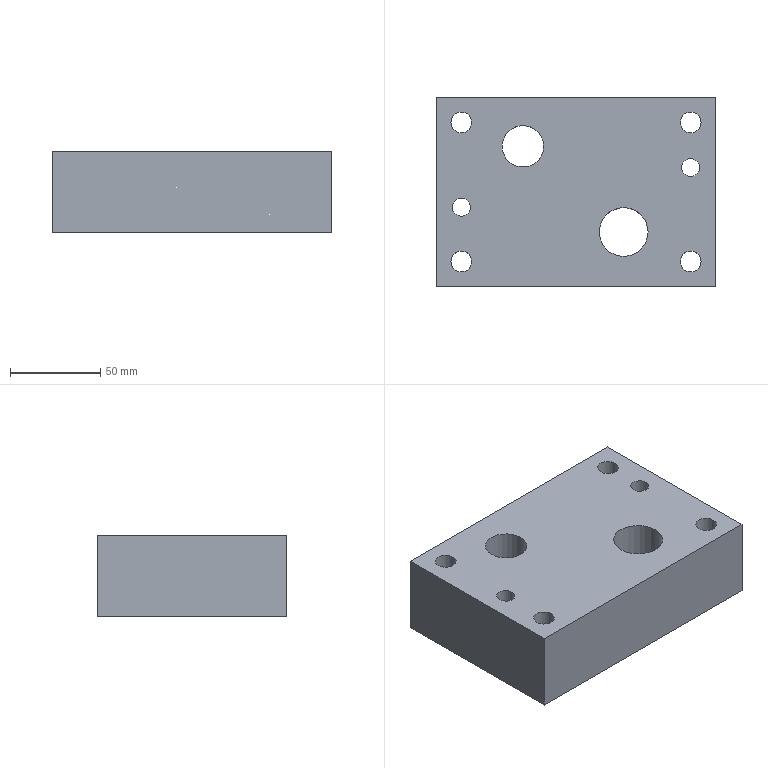Part | STEP file | lll_id4718_x_t | 1 solid | 14 faces | box 155 x 105 x 45 mm | volume 662119 mm3 | cylinder 8 | plane 6 | commonest cylinder face diameters 11.509 x4 10 x2 23 x1 27 x1
STEP:
#1=CARTESIAN_POINT('',(448.5,-300.,-80.));
#2=VERTEX_POINT('',#1);
#3=CARTESIAN_POINT('',(437.,-300.,-80.));
#4=DIRECTION('',(0.,0.,1.));
#5=DIRECTION('',(1.,0.,0.));
#6=AXIS2_PLACEMENT_3D('',#3,#4,#5);
#7=CIRCLE('',#6,11.5);
#8=EDGE_CURVE('',#2,#2,#7,.T.);
#9=ORIENTED_EDGE('',*,*,#8,.T.);
#10=EDGE_LOOP('',(#9));
#11=FACE_BOUND('',#10,.T.);
#12=CARTESIAN_POINT('',(388.935,-377.75,-80.));
#13=VERTEX_POINT('',#12);
#14=CARTESIAN_POINT('',(388.935,-272.75,-80.));
#15=VERTEX_POINT('',#14);
#16=CARTESIAN_POINT('',(388.935,0.,-80.));
#17=DIRECTION('',(0.,1.,0.));
#18=VECTOR('',#17,1.);
#19=LINE('',#16,#18);
#20=EDGE_CURVE('',#13,#15,#19,.T.);
#21=ORIENTED_EDGE('',*,*,#20,.T.);
#22=CARTESIAN_POINT('',(543.935,-272.75,-80.));
#23=VERTEX_POINT('',#22);
#24=CARTESIAN_POINT('',(2132.435,-272.75,-80.));
#25=DIRECTION('',(1.,0.,0.));
#26=VECTOR('',#25,1.);
#27=LINE('',#24,#26);
#28=EDGE_CURVE('',#15,#23,#27,.T.);
#29=ORIENTED_EDGE('',*,*,#28,.T.);
#30=CARTESIAN_POINT('',(543.935,-377.75,-80.));
#31=VERTEX_POINT('',#30);
#32=CARTESIAN_POINT('',(543.935,0.,-80.));
#33=DIRECTION('',(0.,-1.,0.));
#34=VECTOR('',#33,1.);
#35=LINE('',#32,#34);
#36=EDGE_CURVE('',#23,#31,#35,.T.);
#37=ORIENTED_EDGE('',*,*,#36,.T.);
#38=CARTESIAN_POINT('',(2132.435,-377.75,-80.));
#39=DIRECTION('',(-1.,0.,0.));
#40=VECTOR('',#39,1.);
#41=LINE('',#38,#40);
#42=EDGE_CURVE('',#31,#13,#41,.T.);
#43=ORIENTED_EDGE('',*,*,#42,.T.);
#44=EDGE_LOOP('',(#21,#29,#37,#43));
#45=FACE_BOUND('',#44,.T.);
#46=CARTESIAN_POINT('',(535.69,-363.75,-80.));
#47=VERTEX_POINT('',#46);
#48=CARTESIAN_POINT('',(529.935,-363.75,-80.));
#49=DIRECTION('',(0.,0.,1.));
#50=DIRECTION('',(1.,0.,0.));
#51=AXIS2_PLACEMENT_3D('',#48,#49,#50);
#52=CIRCLE('',#51,5.755);
#53=EDGE_CURVE('',#47,#47,#52,.T.);
#54=ORIENTED_EDGE('',*,*,#53,.T.);
#55=EDGE_LOOP('',(#54));
#56=FACE_BOUND('',#55,.T.);
#57=CARTESIAN_POINT('',(535.69,-286.75,-80.));
#58=VERTEX_POINT('',#57);
#59=CARTESIAN_POINT('',(529.935,-286.75,-80.));
#60=DIRECTION('',(0.,0.,1.));
#61=DIRECTION('',(1.,0.,0.));
#62=AXIS2_PLACEMENT_3D('',#59,#60,#61);
#63=CIRCLE('',#62,5.755);
#64=EDGE_CURVE('',#58,#58,#63,.T.);
#65=ORIENTED_EDGE('',*,*,#64,.T.);
#66=EDGE_LOOP('',(#65));
#67=FACE_BOUND('',#66,.T.);
#68=CARTESIAN_POINT('',(534.935,-311.75,-80.));
#69=VERTEX_POINT('',#68);
#70=CARTESIAN_POINT('',(529.935,-311.75,-80.));
#71=DIRECTION('',(0.,0.,1.));
#72=DIRECTION('',(1.,0.,0.));
#73=AXIS2_PLACEMENT_3D('',#70,#71,#72);
#74=CIRCLE('',#73,5.);
#75=EDGE_CURVE('',#69,#69,#74,.T.);
#76=ORIENTED_EDGE('',*,*,#75,.T.);
#77=EDGE_LOOP('',(#76));
#78=FACE_BOUND('',#77,.T.);
#79=CARTESIAN_POINT('',(408.69,-286.75,-80.));
#80=VERTEX_POINT('',#79);
#81=CARTESIAN_POINT('',(402.935,-286.75,-80.));
#82=DIRECTION('',(0.,0.,1.));
#83=DIRECTION('',(1.,0.,0.));
#84=AXIS2_PLACEMENT_3D('',#81,#82,#83);
#85=CIRCLE('',#84,5.755);
#86=EDGE_CURVE('',#80,#80,#85,.T.);
#87=ORIENTED_EDGE('',*,*,#86,.T.);
#88=EDGE_LOOP('',(#87));
#89=FACE_BOUND('',#88,.T.);
#90=CARTESIAN_POINT('',(408.69,-363.75,-80.));
#91=VERTEX_POINT('',#90);
#92=CARTESIAN_POINT('',(402.935,-363.75,-80.));
#93=DIRECTION('',(0.,0.,1.));
#94=DIRECTION('',(1.,0.,0.));
#95=AXIS2_PLACEMENT_3D('',#92,#93,#94);
#96=CIRCLE('',#95,5.755);
#97=EDGE_CURVE('',#91,#91,#96,.T.);
#98=ORIENTED_EDGE('',*,*,#97,.T.);
#99=EDGE_LOOP('',(#98));
#100=FACE_BOUND('',#99,.T.);
#101=CARTESIAN_POINT('',(407.935,-333.75,-80.));
#102=VERTEX_POINT('',#101);
#103=CARTESIAN_POINT('',(402.935,-333.75,-80.));
#104=DIRECTION('',(0.,0.,1.));
#105=DIRECTION('',(1.,0.,0.));
#106=AXIS2_PLACEMENT_3D('',#103,#104,#105);
#107=CIRCLE('',#106,5.);
#108=EDGE_CURVE('',#102,#102,#107,.T.);
#109=ORIENTED_EDGE('',*,*,#108,.T.);
#110=EDGE_LOOP('',(#109));
#111=FACE_BOUND('',#110,.T.);
#112=CARTESIAN_POINT('',(506.37,-347.42,-80.));
#113=VERTEX_POINT('',#112);
#114=CARTESIAN_POINT('',(492.87,-347.42,-80.));
#115=DIRECTION('',(0.,0.,1.));
#116=DIRECTION('',(1.,0.,0.));
#117=AXIS2_PLACEMENT_3D('',#114,#115,#116);
#118=CIRCLE('',#117,13.5);
#119=EDGE_CURVE('',#113,#113,#118,.T.);
#120=ORIENTED_EDGE('',*,*,#119,.T.);
#121=EDGE_LOOP('',(#120));
#122=FACE_BOUND('',#121,.T.);
#123=CARTESIAN_POINT('',(2132.435,0.,-80.));
#124=DIRECTION('',(0.,0.,1.));
#125=DIRECTION('',(1.,0.,0.));
#126=AXIS2_PLACEMENT_3D('',#123,#124,#125);
#127=PLANE('',#126);
#128=ADVANCED_FACE('',(#11,#45,#56,#67,#78,#89,#100,#111,#122),#127,.F.);
#129=CARTESIAN_POINT('',(543.935,-272.75,-35.));
#130=VERTEX_POINT('',#129);
#131=CARTESIAN_POINT('',(543.935,-272.75,-35.));
#132=DIRECTION('',(0.,0.,-1.));
#133=VECTOR('',#132,1.);
#134=LINE('',#131,#133);
#135=EDGE_CURVE('',#130,#23,#134,.T.);
#136=ORIENTED_EDGE('',*,*,#135,.F.);
#137=CARTESIAN_POINT('',(543.935,-377.75,-35.));
#138=VERTEX_POINT('',#137);
#139=CARTESIAN_POINT('',(543.935,-325.25,-35.));
#140=DIRECTION('',(0.,-1.,0.));
#141=VECTOR('',#140,1.);
#142=LINE('',#139,#141);
#143=EDGE_CURVE('',#130,#138,#142,.T.);
#144=ORIENTED_EDGE('',*,*,#143,.T.);
#145=CARTESIAN_POINT('',(543.935,-377.75,-35.));
#146=DIRECTION('',(0.,0.,-1.));
#147=VECTOR('',#146,1.);
#148=LINE('',#145,#147);
#149=EDGE_CURVE('',#138,#31,#148,.T.);
#150=ORIENTED_EDGE('',*,*,#149,.T.);
#151=ORIENTED_EDGE('',*,*,#36,.F.);
#152=EDGE_LOOP('',(#136,#144,#150,#151));
#153=FACE_OUTER_BOUND('',#152,.T.);
#154=CARTESIAN_POINT('',(543.935,-325.25,-35.));
#155=DIRECTION('',(1.,0.,0.));
#156=DIRECTION('',(0.,-1.,0.));
#157=AXIS2_PLACEMENT_3D('',#154,#155,#156);
#158=PLANE('',#157);
#159=ADVANCED_FACE('',(#153),#158,.T.);
#160=ORIENTED_EDGE('',*,*,#149,.F.);
#161=CARTESIAN_POINT('',(388.935,-377.75,-35.));
#162=VERTEX_POINT('',#161);
#163=CARTESIAN_POINT('',(466.435,-377.75,-35.));
#164=DIRECTION('',(-1.,0.,0.));
#165=VECTOR('',#164,1.);
#166=LINE('',#163,#165);
#167=EDGE_CURVE('',#138,#162,#166,.T.);
#168=ORIENTED_EDGE('',*,*,#167,.T.);
#169=CARTESIAN_POINT('',(388.935,-377.75,-35.));
#170=DIRECTION('',(0.,0.,-1.));
#171=VECTOR('',#170,1.);
#172=LINE('',#169,#171);
#173=EDGE_CURVE('',#162,#13,#172,.T.);
#174=ORIENTED_EDGE('',*,*,#173,.T.);
#175=ORIENTED_EDGE('',*,*,#42,.F.);
#176=EDGE_LOOP('',(#160,#168,#174,#175));
#177=FACE_OUTER_BOUND('',#176,.T.);
#178=CARTESIAN_POINT('',(466.435,-377.75,-35.));
#179=DIRECTION('',(0.,-1.,0.));
#180=DIRECTION('',(-1.,0.,0.));
#181=AXIS2_PLACEMENT_3D('',#178,#179,#180);
#182=PLANE('',#181);
#183=ADVANCED_FACE('',(#177),#182,.T.);
#184=ORIENTED_EDGE('',*,*,#173,.F.);
#185=CARTESIAN_POINT('',(388.935,-272.75,-35.));
#186=VERTEX_POINT('',#185);
#187=CARTESIAN_POINT('',(388.935,-325.25,-35.));
#188=DIRECTION('',(0.,1.,0.));
#189=VECTOR('',#188,1.);
#190=LINE('',#187,#189);
#191=EDGE_CURVE('',#162,#186,#190,.T.);
#192=ORIENTED_EDGE('',*,*,#191,.T.);
#193=CARTESIAN_POINT('',(388.935,-272.75,-35.));
#194=DIRECTION('',(0.,0.,-1.));
#195=VECTOR('',#194,1.);
#196=LINE('',#193,#195);
#197=EDGE_CURVE('',#186,#15,#196,.T.);
#198=ORIENTED_EDGE('',*,*,#197,.T.);
#199=ORIENTED_EDGE('',*,*,#20,.F.);
#200=EDGE_LOOP('',(#184,#192,#198,#199));
#201=FACE_OUTER_BOUND('',#200,.T.);
#202=CARTESIAN_POINT('',(388.935,-325.25,-35.));
#203=DIRECTION('',(-1.,0.,0.));
#204=DIRECTION('',(0.,1.,0.));
#205=AXIS2_PLACEMENT_3D('',#202,#203,#204);
#206=PLANE('',#205);
#207=ADVANCED_FACE('',(#201),#206,.T.);
#208=CARTESIAN_POINT('',(466.435,-272.75,-35.));
#209=DIRECTION('',(1.,0.,0.));
#210=VECTOR('',#209,1.);
#211=LINE('',#208,#210);
#212=EDGE_CURVE('',#186,#130,#211,.T.);
#213=ORIENTED_EDGE('',*,*,#212,.T.);
#214=ORIENTED_EDGE('',*,*,#135,.T.);
#215=ORIENTED_EDGE('',*,*,#28,.F.);
#216=ORIENTED_EDGE('',*,*,#197,.F.);
#217=EDGE_LOOP('',(#213,#214,#215,#216));
#218=FACE_OUTER_BOUND('',#217,.T.);
#219=CARTESIAN_POINT('',(466.435,-272.75,-35.));
#220=DIRECTION('',(0.,1.,0.));
#221=DIRECTION('',(1.,0.,0.));
#222=AXIS2_PLACEMENT_3D('',#219,#220,#221);
#223=PLANE('',#222);
#224=ADVANCED_FACE('',(#218),#223,.T.);
#225=ORIENTED_EDGE('',*,*,#53,.F.);
#226=EDGE_LOOP('',(#225));
#227=FACE_BOUND('',#226,.T.);
#228=CARTESIAN_POINT('',(535.69,-363.75,-35.));
#229=VERTEX_POINT('',#228);
#230=CARTESIAN_POINT('',(529.935,-363.75,-35.));
#231=DIRECTION('',(0.,0.,1.));
#232=DIRECTION('',(1.,0.,0.));
#233=AXIS2_PLACEMENT_3D('',#230,#231,#232);
#234=CIRCLE('',#233,5.755);
#235=EDGE_CURVE('',#229,#229,#234,.T.);
#236=ORIENTED_EDGE('',*,*,#235,.T.);
#237=EDGE_LOOP('',(#236));
#238=FACE_BOUND('',#237,.T.);
#239=CARTESIAN_POINT('',(529.935,-363.75,-35.));
#240=DIRECTION('',(0.,0.,1.));
#241=DIRECTION('',(1.,0.,0.));
#242=AXIS2_PLACEMENT_3D('',#239,#240,#241);
#243=CYLINDRICAL_SURFACE('',#242,5.755);
#244=ADVANCED_FACE('',(#227,#238),#243,.F.);
#245=ORIENTED_EDGE('',*,*,#64,.F.);
#246=EDGE_LOOP('',(#245));
#247=FACE_BOUND('',#246,.T.);
#248=CARTESIAN_POINT('',(535.69,-286.75,-35.));
#249=VERTEX_POINT('',#248);
#250=CARTESIAN_POINT('',(529.935,-286.75,-35.));
#251=DIRECTION('',(0.,0.,1.));
#252=DIRECTION('',(1.,0.,0.));
#253=AXIS2_PLACEMENT_3D('',#250,#251,#252);
#254=CIRCLE('',#253,5.755);
#255=EDGE_CURVE('',#249,#249,#254,.T.);
#256=ORIENTED_EDGE('',*,*,#255,.T.);
#257=EDGE_LOOP('',(#256));
#258=FACE_BOUND('',#257,.T.);
#259=CARTESIAN_POINT('',(529.935,-286.75,-35.));
#260=DIRECTION('',(0.,0.,1.));
#261=DIRECTION('',(1.,0.,0.));
#262=AXIS2_PLACEMENT_3D('',#259,#260,#261);
#263=CYLINDRICAL_SURFACE('',#262,5.755);
#264=ADVANCED_FACE('',(#247,#258),#263,.F.);
#265=ORIENTED_EDGE('',*,*,#75,.F.);
#266=EDGE_LOOP('',(#265));
#267=FACE_BOUND('',#266,.T.);
#268=CARTESIAN_POINT('',(534.935,-311.75,-35.));
#269=VERTEX_POINT('',#268);
#270=CARTESIAN_POINT('',(529.935,-311.75,-35.));
#271=DIRECTION('',(0.,0.,1.));
#272=DIRECTION('',(1.,0.,0.));
#273=AXIS2_PLACEMENT_3D('',#270,#271,#272);
#274=CIRCLE('',#273,5.);
#275=EDGE_CURVE('',#269,#269,#274,.T.);
#276=ORIENTED_EDGE('',*,*,#275,.T.);
#277=EDGE_LOOP('',(#276));
#278=FACE_BOUND('',#277,.T.);
#279=CARTESIAN_POINT('',(529.935,-311.75,-35.));
#280=DIRECTION('',(0.,0.,1.));
#281=DIRECTION('',(1.,0.,0.));
#282=AXIS2_PLACEMENT_3D('',#279,#280,#281);
#283=CYLINDRICAL_SURFACE('',#282,5.);
#284=ADVANCED_FACE('',(#267,#278),#283,.F.);
#285=ORIENTED_EDGE('',*,*,#86,.F.);
#286=EDGE_LOOP('',(#285));
#287=FACE_BOUND('',#286,.T.);
#288=CARTESIAN_POINT('',(408.69,-286.75,-35.));
#289=VERTEX_POINT('',#288);
#290=CARTESIAN_POINT('',(402.935,-286.75,-35.));
#291=DIRECTION('',(0.,0.,1.));
#292=DIRECTION('',(1.,0.,0.));
#293=AXIS2_PLACEMENT_3D('',#290,#291,#292);
#294=CIRCLE('',#293,5.755);
#295=EDGE_CURVE('',#289,#289,#294,.T.);
#296=ORIENTED_EDGE('',*,*,#295,.T.);
#297=EDGE_LOOP('',(#296));
#298=FACE_BOUND('',#297,.T.);
#299=CARTESIAN_POINT('',(402.935,-286.75,-35.));
#300=DIRECTION('',(0.,0.,1.));
#301=DIRECTION('',(1.,0.,0.));
#302=AXIS2_PLACEMENT_3D('',#299,#300,#301);
#303=CYLINDRICAL_SURFACE('',#302,5.755);
#304=ADVANCED_FACE('',(#287,#298),#303,.F.);
#305=ORIENTED_EDGE('',*,*,#97,.F.);
#306=EDGE_LOOP('',(#305));
#307=FACE_BOUND('',#306,.T.);
#308=CARTESIAN_POINT('',(408.69,-363.75,-35.));
#309=VERTEX_POINT('',#308);
#310=CARTESIAN_POINT('',(402.935,-363.75,-35.));
#311=DIRECTION('',(0.,0.,1.));
#312=DIRECTION('',(1.,0.,0.));
#313=AXIS2_PLACEMENT_3D('',#310,#311,#312);
#314=CIRCLE('',#313,5.755);
#315=EDGE_CURVE('',#309,#309,#314,.T.);
#316=ORIENTED_EDGE('',*,*,#315,.T.);
#317=EDGE_LOOP('',(#316));
#318=FACE_BOUND('',#317,.T.);
#319=CARTESIAN_POINT('',(402.935,-363.75,-35.));
#320=DIRECTION('',(0.,0.,1.));
#321=DIRECTION('',(1.,0.,0.));
#322=AXIS2_PLACEMENT_3D('',#319,#320,#321);
#323=CYLINDRICAL_SURFACE('',#322,5.755);
#324=ADVANCED_FACE('',(#307,#318),#323,.F.);
#325=ORIENTED_EDGE('',*,*,#108,.F.);
#326=EDGE_LOOP('',(#325));
#327=FACE_BOUND('',#326,.T.);
#328=CARTESIAN_POINT('',(407.935,-333.75,-35.));
#329=VERTEX_POINT('',#328);
#330=CARTESIAN_POINT('',(402.935,-333.75,-35.));
#331=DIRECTION('',(0.,0.,1.));
#332=DIRECTION('',(1.,0.,0.));
#333=AXIS2_PLACEMENT_3D('',#330,#331,#332);
#334=CIRCLE('',#333,5.);
#335=EDGE_CURVE('',#329,#329,#334,.T.);
#336=ORIENTED_EDGE('',*,*,#335,.T.);
#337=EDGE_LOOP('',(#336));
#338=FACE_BOUND('',#337,.T.);
#339=CARTESIAN_POINT('',(402.935,-333.75,-35.));
#340=DIRECTION('',(0.,0.,1.));
#341=DIRECTION('',(1.,0.,0.));
#342=AXIS2_PLACEMENT_3D('',#339,#340,#341);
#343=CYLINDRICAL_SURFACE('',#342,5.);
#344=ADVANCED_FACE('',(#327,#338),#343,.F.);
#345=CARTESIAN_POINT('',(479.37,-347.42,-35.));
#346=VERTEX_POINT('',#345);
#347=CARTESIAN_POINT('',(492.87,-347.42,-35.));
#348=DIRECTION('',(0.,0.,-1.));
#349=DIRECTION('',(-1.,0.,0.));
#350=AXIS2_PLACEMENT_3D('',#347,#348,#349);
#351=CIRCLE('',#350,13.5);
#352=EDGE_CURVE('',#346,#346,#351,.T.);
#353=ORIENTED_EDGE('',*,*,#352,.T.);
#354=EDGE_LOOP('',(#353));
#355=FACE_BOUND('',#354,.T.);
#356=CARTESIAN_POINT('',(425.5,-300.,-35.));
#357=VERTEX_POINT('',#356);
#358=CARTESIAN_POINT('',(437.,-300.,-35.));
#359=DIRECTION('',(0.,0.,-1.));
#360=DIRECTION('',(-1.,0.,0.));
#361=AXIS2_PLACEMENT_3D('',#358,#359,#360);
#362=CIRCLE('',#361,11.5);
#363=EDGE_CURVE('',#357,#357,#362,.T.);
#364=ORIENTED_EDGE('',*,*,#363,.T.);
#365=EDGE_LOOP('',(#364));
#366=FACE_BOUND('',#365,.T.);
#367=ORIENTED_EDGE('',*,*,#191,.F.);
#368=ORIENTED_EDGE('',*,*,#167,.F.);
#369=ORIENTED_EDGE('',*,*,#143,.F.);
#370=ORIENTED_EDGE('',*,*,#212,.F.);
#371=EDGE_LOOP('',(#367,#368,#369,#370));
#372=FACE_BOUND('',#371,.T.);
#373=ORIENTED_EDGE('',*,*,#235,.F.);
#374=EDGE_LOOP('',(#373));
#375=FACE_BOUND('',#374,.T.);
#376=ORIENTED_EDGE('',*,*,#255,.F.);
#377=EDGE_LOOP('',(#376));
#378=FACE_BOUND('',#377,.T.);
#379=ORIENTED_EDGE('',*,*,#275,.F.);
#380=EDGE_LOOP('',(#379));
#381=FACE_BOUND('',#380,.T.);
#382=ORIENTED_EDGE('',*,*,#295,.F.);
#383=EDGE_LOOP('',(#382));
#384=FACE_BOUND('',#383,.T.);
#385=ORIENTED_EDGE('',*,*,#315,.F.);
#386=EDGE_LOOP('',(#385));
#387=FACE_BOUND('',#386,.T.);
#388=ORIENTED_EDGE('',*,*,#335,.F.);
#389=EDGE_LOOP('',(#388));
#390=FACE_BOUND('',#389,.T.);
#391=CARTESIAN_POINT('',(466.435,-325.25,-35.));
#392=DIRECTION('',(0.,0.,-1.));
#393=DIRECTION('',(1.,0.,0.));
#394=AXIS2_PLACEMENT_3D('',#391,#392,#393);
#395=PLANE('',#394);
#396=ADVANCED_FACE('',(#355,#366,#372,#375,#378,#381,#384,#387,#390),#395,.F.);
#397=ORIENTED_EDGE('',*,*,#8,.F.);
#398=EDGE_LOOP('',(#397));
#399=FACE_BOUND('',#398,.T.);
#400=ORIENTED_EDGE('',*,*,#363,.F.);
#401=EDGE_LOOP('',(#400));
#402=FACE_BOUND('',#401,.T.);
#403=CARTESIAN_POINT('',(437.,-300.,-120.));
#404=DIRECTION('',(0.,0.,1.));
#405=DIRECTION('',(1.,0.,0.));
#406=AXIS2_PLACEMENT_3D('',#403,#404,#405);
#407=CYLINDRICAL_SURFACE('',#406,11.5);
#408=ADVANCED_FACE('',(#399,#402),#407,.F.);
#409=ORIENTED_EDGE('',*,*,#119,.F.);
#410=EDGE_LOOP('',(#409));
#411=FACE_BOUND('',#410,.T.);
#412=ORIENTED_EDGE('',*,*,#352,.F.);
#413=EDGE_LOOP('',(#412));
#414=FACE_BOUND('',#413,.T.);
#415=CARTESIAN_POINT('',(492.87,-347.42,-120.));
#416=DIRECTION('',(0.,0.,1.));
#417=DIRECTION('',(1.,0.,0.));
#418=AXIS2_PLACEMENT_3D('',#415,#416,#417);
#419=CYLINDRICAL_SURFACE('',#418,13.5);
#420=ADVANCED_FACE('',(#411,#414),#419,.F.);
#421=CLOSED_SHELL('',(#128,#159,#183,#207,#224,#244,#264,#284,#304,#324,#344,#396,#408,#420));
#422=MANIFOLD_SOLID_BREP('',#421);
#423=(LENGTH_UNIT()NAMED_UNIT(*)SI_UNIT(.MILLI.,.METRE.));
#424=UNCERTAINTY_MEASURE_WITH_UNIT(LENGTH_MEASURE(0.00002),#423,'','');
#425=(NAMED_UNIT(*)PLANE_ANGLE_UNIT()SI_UNIT($,.RADIAN.));
#426=PLANE_ANGLE_MEASURE_WITH_UNIT(PLANE_ANGLE_MEASURE(0.01745),#425);
#427=DIMENSIONAL_EXPONENTS(0.,0.,0.,0.,0.,0.,0.);
#428=(CONVERSION_BASED_UNIT('DEGREE',#426)NAMED_UNIT(#427)PLANE_ANGLE_UNIT());
#429=(NAMED_UNIT(*)SI_UNIT($,.STERADIAN.)SOLID_ANGLE_UNIT());
#430=(GEOMETRIC_REPRESENTATION_CONTEXT(3)GLOBAL_UNCERTAINTY_ASSIGNED_CONTEXT((#424))GLOBAL_UNIT_ASSIGNED_CONTEXT((#423,#428,#429))REPRESENTATION_CONTEXT('',''));
#431=ADVANCED_BREP_SHAPE_REPRESENTATION('',(#422),#430);